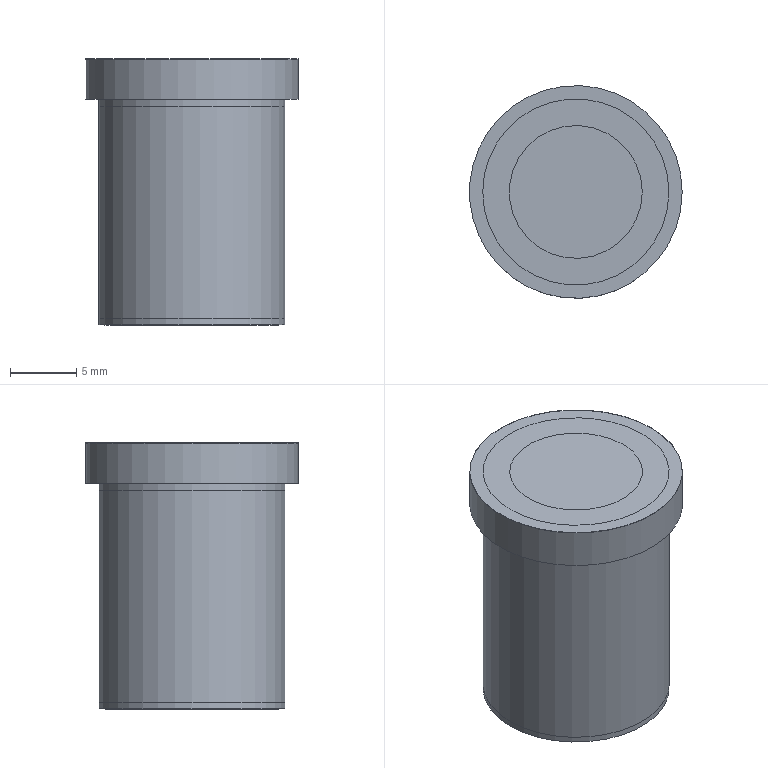Part | NX | features BREP 2 | 2 solids | 16 faces | box 16 x 16 x 20.03 mm | volume 4861 mm3 | plane 8 | cylinder 7 | cone 1 | commonest cylinder face diameters 14 x3 16 x2 10 x1 13.533 x1
STEP:
#1=CARTESIAN_POINT('',(8.,0.,-3.03));
#2=VERTEX_POINT('',#1);
#3=CARTESIAN_POINT('',(0.,0.,-3.03));
#4=DIRECTION('',(0.,0.,1.));
#5=DIRECTION('',(1.,0.,0.));
#6=AXIS2_PLACEMENT_3D('',#3,#4,#5);
#7=CIRCLE('',#6,8.);
#8=EDGE_CURVE('',#2,#2,#7,.T.);
#9=ORIENTED_EDGE('',*,*,#8,.T.);
#10=EDGE_LOOP('',(#9));
#11=FACE_BOUND('',#10,.T.);
#12=CARTESIAN_POINT('',(8.,0.,0.));
#13=VERTEX_POINT('',#12);
#14=CARTESIAN_POINT('',(0.,0.,0.));
#15=DIRECTION('',(0.,0.,1.));
#16=DIRECTION('',(1.,0.,0.));
#17=AXIS2_PLACEMENT_3D('',#14,#15,#16);
#18=CIRCLE('',#17,8.);
#19=EDGE_CURVE('',#13,#13,#18,.T.);
#20=ORIENTED_EDGE('',*,*,#19,.F.);
#21=EDGE_LOOP('',(#20));
#22=FACE_BOUND('',#21,.T.);
#23=CARTESIAN_POINT('',(0.,0.,-3.03));
#24=DIRECTION('',(0.,0.,1.));
#25=DIRECTION('',(-1.,0.,0.));
#26=AXIS2_PLACEMENT_3D('',#23,#24,#25);
#27=CYLINDRICAL_SURFACE('',#26,8.);
#28=ADVANCED_FACE('',(#11,#22),#27,.T.);
#29=CARTESIAN_POINT('',(-7.,0.,-3.03));
#30=VERTEX_POINT('',#29);
#31=CARTESIAN_POINT('',(0.,0.,-3.03));
#32=DIRECTION('',(0.,0.,-1.));
#33=DIRECTION('',(-1.,0.,0.));
#34=AXIS2_PLACEMENT_3D('',#31,#32,#33);
#35=CIRCLE('',#34,7.);
#36=EDGE_CURVE('',#30,#30,#35,.T.);
#37=ORIENTED_EDGE('',*,*,#36,.F.);
#38=EDGE_LOOP('',(#37));
#39=FACE_BOUND('',#38,.T.);
#40=ORIENTED_EDGE('',*,*,#8,.F.);
#41=EDGE_LOOP('',(#40));
#42=FACE_BOUND('',#41,.T.);
#43=CARTESIAN_POINT('',(0.,0.,-3.03));
#44=DIRECTION('',(0.,0.,1.));
#45=DIRECTION('',(-1.,0.,0.));
#46=AXIS2_PLACEMENT_3D('',#43,#44,#45);
#47=PLANE('',#46);
#48=ADVANCED_FACE('',(#39,#42),#47,.F.);
#49=ORIENTED_EDGE('',*,*,#19,.T.);
#50=EDGE_LOOP('',(#49));
#51=FACE_BOUND('',#50,.T.);
#52=CARTESIAN_POINT('',(0.,0.,0.));
#53=DIRECTION('',(0.,0.,1.));
#54=DIRECTION('',(-1.,0.,0.));
#55=AXIS2_PLACEMENT_3D('',#52,#53,#54);
#56=PLANE('',#55);
#57=ADVANCED_FACE('',(#51),#56,.T.);
#58=CARTESIAN_POINT('',(-7.,0.,-20.));
#59=VERTEX_POINT('',#58);
#60=CARTESIAN_POINT('',(0.,0.,-20.));
#61=DIRECTION('',(0.,0.,-1.));
#62=DIRECTION('',(-1.,0.,0.));
#63=AXIS2_PLACEMENT_3D('',#60,#61,#62);
#64=CIRCLE('',#63,7.);
#65=EDGE_CURVE('',#59,#59,#64,.T.);
#66=ORIENTED_EDGE('',*,*,#65,.T.);
#67=EDGE_LOOP('',(#66));
#68=FACE_BOUND('',#67,.T.);
#69=CARTESIAN_POINT('',(0.,0.,-20.));
#70=DIRECTION('',(0.,0.,-1.));
#71=DIRECTION('',(1.,0.,0.));
#72=AXIS2_PLACEMENT_3D('',#69,#70,#71);
#73=PLANE('',#72);
#74=ADVANCED_FACE('',(#68),#73,.T.);
#75=ORIENTED_EDGE('',*,*,#65,.F.);
#76=EDGE_LOOP('',(#75));
#77=FACE_BOUND('',#76,.T.);
#78=ORIENTED_EDGE('',*,*,#36,.T.);
#79=EDGE_LOOP('',(#78));
#80=FACE_BOUND('',#79,.T.);
#81=CARTESIAN_POINT('',(0.,0.,-3.03));
#82=DIRECTION('',(0.,0.,-1.));
#83=DIRECTION('',(1.,0.,0.));
#84=AXIS2_PLACEMENT_3D('',#81,#82,#83);
#85=CYLINDRICAL_SURFACE('',#84,7.);
#86=ADVANCED_FACE('',(#77,#80),#85,.T.);
#87=CLOSED_SHELL('',(#28,#48,#57,#74,#86));
#88=MANIFOLD_SOLID_BREP('',#87);
#89=CARTESIAN_POINT('',(-6.533,0.,-20.03));
#90=VERTEX_POINT('',#89);
#91=CARTESIAN_POINT('',(0.,0.,-20.03));
#92=DIRECTION('',(0.,0.,-1.));
#93=DIRECTION('',(-1.,0.,0.));
#94=AXIS2_PLACEMENT_3D('',#91,#92,#93);
#95=CIRCLE('',#94,6.533);
#96=EDGE_CURVE('',#90,#90,#95,.T.);
#97=ORIENTED_EDGE('',*,*,#96,.T.);
#98=EDGE_LOOP('',(#97));
#99=FACE_BOUND('',#98,.T.);
#100=CARTESIAN_POINT('',(5.,0.,-20.03));
#101=VERTEX_POINT('',#100);
#102=CARTESIAN_POINT('',(0.,0.,-20.03));
#103=DIRECTION('',(0.,0.,1.));
#104=DIRECTION('',(1.,0.,0.));
#105=AXIS2_PLACEMENT_3D('',#102,#103,#104);
#106=CIRCLE('',#105,5.);
#107=EDGE_CURVE('',#101,#101,#106,.T.);
#108=ORIENTED_EDGE('',*,*,#107,.T.);
#109=EDGE_LOOP('',(#108));
#110=FACE_BOUND('',#109,.T.);
#111=CARTESIAN_POINT('',(0.,0.,-20.03));
#112=DIRECTION('',(0.,0.,-1.));
#113=DIRECTION('',(1.,0.,0.));
#114=AXIS2_PLACEMENT_3D('',#111,#112,#113);
#115=PLANE('',#114);
#116=ADVANCED_FACE('',(#99,#110),#115,.T.);
#117=CARTESIAN_POINT('',(7.,0.,-0.026));
#118=VERTEX_POINT('',#117);
#119=CARTESIAN_POINT('',(0.,0.,-0.026));
#120=DIRECTION('',(0.,0.,1.));
#121=DIRECTION('',(1.,0.,0.));
#122=AXIS2_PLACEMENT_3D('',#119,#120,#121);
#123=CIRCLE('',#122,7.);
#124=EDGE_CURVE('',#118,#118,#123,.T.);
#125=ORIENTED_EDGE('',*,*,#124,.T.);
#126=EDGE_LOOP('',(#125));
#127=FACE_BOUND('',#126,.T.);
#128=CARTESIAN_POINT('',(5.,0.,-0.026));
#129=VERTEX_POINT('',#128);
#130=CARTESIAN_POINT('',(0.,0.,-0.026));
#131=DIRECTION('',(0.,0.,1.));
#132=DIRECTION('',(1.,0.,0.));
#133=AXIS2_PLACEMENT_3D('',#130,#131,#132);
#134=CIRCLE('',#133,5.);
#135=EDGE_CURVE('',#129,#129,#134,.T.);
#136=ORIENTED_EDGE('',*,*,#135,.F.);
#137=EDGE_LOOP('',(#136));
#138=FACE_BOUND('',#137,.T.);
#139=CARTESIAN_POINT('',(0.,0.,-0.026));
#140=DIRECTION('',(0.,0.,1.));
#141=DIRECTION('',(-1.,0.,0.));
#142=AXIS2_PLACEMENT_3D('',#139,#140,#141);
#143=PLANE('',#142);
#144=ADVANCED_FACE('',(#127,#138),#143,.T.);
#145=CARTESIAN_POINT('',(8.,0.,-3.03));
#146=VERTEX_POINT('',#145);
#147=CARTESIAN_POINT('',(0.,0.,-3.03));
#148=DIRECTION('',(0.,0.,1.));
#149=DIRECTION('',(1.,0.,0.));
#150=AXIS2_PLACEMENT_3D('',#147,#148,#149);
#151=CIRCLE('',#150,8.);
#152=EDGE_CURVE('',#146,#146,#151,.T.);
#153=ORIENTED_EDGE('',*,*,#152,.T.);
#154=EDGE_LOOP('',(#153));
#155=FACE_BOUND('',#154,.T.);
#156=CARTESIAN_POINT('',(8.,0.,-0.03));
#157=VERTEX_POINT('',#156);
#158=CARTESIAN_POINT('',(0.,0.,-0.03));
#159=DIRECTION('',(0.,0.,1.));
#160=DIRECTION('',(1.,0.,0.));
#161=AXIS2_PLACEMENT_3D('',#158,#159,#160);
#162=CIRCLE('',#161,8.);
#163=EDGE_CURVE('',#157,#157,#162,.T.);
#164=ORIENTED_EDGE('',*,*,#163,.F.);
#165=EDGE_LOOP('',(#164));
#166=FACE_BOUND('',#165,.T.);
#167=CARTESIAN_POINT('',(0.,0.,-3.03));
#168=DIRECTION('',(0.,0.,1.));
#169=DIRECTION('',(-1.,0.,0.));
#170=AXIS2_PLACEMENT_3D('',#167,#168,#169);
#171=CYLINDRICAL_SURFACE('',#170,8.);
#172=ADVANCED_FACE('',(#155,#166),#171,.T.);
#173=ORIENTED_EDGE('',*,*,#152,.F.);
#174=EDGE_LOOP('',(#173));
#175=FACE_BOUND('',#174,.T.);
#176=CARTESIAN_POINT('',(-6.767,0.,-3.03));
#177=VERTEX_POINT('',#176);
#178=CARTESIAN_POINT('',(0.,0.,-3.03));
#179=DIRECTION('',(0.,0.,-1.));
#180=DIRECTION('',(-1.,0.,0.));
#181=AXIS2_PLACEMENT_3D('',#178,#179,#180);
#182=CIRCLE('',#181,6.767);
#183=EDGE_CURVE('',#177,#177,#182,.T.);
#184=ORIENTED_EDGE('',*,*,#183,.F.);
#185=EDGE_LOOP('',(#184));
#186=FACE_BOUND('',#185,.T.);
#187=CARTESIAN_POINT('',(0.,0.,-3.03));
#188=DIRECTION('',(0.,0.,1.));
#189=DIRECTION('',(-1.,0.,0.));
#190=AXIS2_PLACEMENT_3D('',#187,#188,#189);
#191=PLANE('',#190);
#192=ADVANCED_FACE('',(#175,#186),#191,.F.);
#193=CARTESIAN_POINT('',(7.,0.,-0.03));
#194=VERTEX_POINT('',#193);
#195=CARTESIAN_POINT('',(0.,0.,-0.03));
#196=DIRECTION('',(0.,0.,1.));
#197=DIRECTION('',(1.,0.,0.));
#198=AXIS2_PLACEMENT_3D('',#195,#196,#197);
#199=CIRCLE('',#198,7.);
#200=EDGE_CURVE('',#194,#194,#199,.T.);
#201=ORIENTED_EDGE('',*,*,#200,.F.);
#202=EDGE_LOOP('',(#201));
#203=FACE_BOUND('',#202,.T.);
#204=ORIENTED_EDGE('',*,*,#163,.T.);
#205=EDGE_LOOP('',(#204));
#206=FACE_BOUND('',#205,.T.);
#207=CARTESIAN_POINT('',(0.,0.,-0.03));
#208=DIRECTION('',(0.,0.,1.));
#209=DIRECTION('',(-1.,0.,0.));
#210=AXIS2_PLACEMENT_3D('',#207,#208,#209);
#211=PLANE('',#210);
#212=ADVANCED_FACE('',(#203,#206),#211,.T.);
#213=CARTESIAN_POINT('',(-7.,0.,-19.563));
#214=VERTEX_POINT('',#213);
#215=CARTESIAN_POINT('',(0.,0.,-19.563));
#216=DIRECTION('',(0.,0.,1.));
#217=DIRECTION('',(-1.,0.,0.));
#218=AXIS2_PLACEMENT_3D('',#215,#216,#217);
#219=CIRCLE('',#218,7.);
#220=EDGE_CURVE('',#214,#214,#219,.T.);
#221=ORIENTED_EDGE('',*,*,#220,.T.);
#222=EDGE_LOOP('',(#221));
#223=FACE_BOUND('',#222,.T.);
#224=CARTESIAN_POINT('',(-7.,0.,-3.59));
#225=VERTEX_POINT('',#224);
#226=CARTESIAN_POINT('',(0.,0.,-3.59));
#227=DIRECTION('',(0.,0.,1.));
#228=DIRECTION('',(-1.,0.,0.));
#229=AXIS2_PLACEMENT_3D('',#226,#227,#228);
#230=CIRCLE('',#229,7.);
#231=EDGE_CURVE('',#225,#225,#230,.T.);
#232=ORIENTED_EDGE('',*,*,#231,.F.);
#233=EDGE_LOOP('',(#232));
#234=FACE_BOUND('',#233,.T.);
#235=CARTESIAN_POINT('',(0.,0.,-3.03));
#236=DIRECTION('',(0.,0.,-1.));
#237=DIRECTION('',(1.,0.,0.));
#238=AXIS2_PLACEMENT_3D('',#235,#236,#237);
#239=CYLINDRICAL_SURFACE('',#238,7.);
#240=ADVANCED_FACE('',(#223,#234),#239,.T.);
#241=ORIENTED_EDGE('',*,*,#124,.F.);
#242=EDGE_LOOP('',(#241));
#243=FACE_BOUND('',#242,.T.);
#244=ORIENTED_EDGE('',*,*,#200,.T.);
#245=EDGE_LOOP('',(#244));
#246=FACE_BOUND('',#245,.T.);
#247=CARTESIAN_POINT('',(0.,0.,-0.03));
#248=DIRECTION('',(0.,0.,1.));
#249=DIRECTION('',(-1.,0.,0.));
#250=AXIS2_PLACEMENT_3D('',#247,#248,#249);
#251=CYLINDRICAL_SURFACE('',#250,7.);
#252=ADVANCED_FACE('',(#243,#246),#251,.T.);
#253=ORIENTED_EDGE('',*,*,#135,.T.);
#254=EDGE_LOOP('',(#253));
#255=FACE_BOUND('',#254,.T.);
#256=ORIENTED_EDGE('',*,*,#107,.F.);
#257=EDGE_LOOP('',(#256));
#258=FACE_BOUND('',#257,.T.);
#259=CARTESIAN_POINT('',(0.,0.,-0.026));
#260=DIRECTION('',(0.,0.,-1.));
#261=DIRECTION('',(1.,0.,0.));
#262=AXIS2_PLACEMENT_3D('',#259,#260,#261);
#263=CYLINDRICAL_SURFACE('',#262,5.);
#264=ADVANCED_FACE('',(#255,#258),#263,.F.);
#265=CARTESIAN_POINT('',(-6.767,0.,-3.59));
#266=VERTEX_POINT('',#265);
#267=CARTESIAN_POINT('',(0.,0.,-3.59));
#268=DIRECTION('',(0.,0.,-1.));
#269=DIRECTION('',(-1.,0.,0.));
#270=AXIS2_PLACEMENT_3D('',#267,#268,#269);
#271=CIRCLE('',#270,6.767);
#272=EDGE_CURVE('',#266,#266,#271,.T.);
#273=ORIENTED_EDGE('',*,*,#272,.F.);
#274=EDGE_LOOP('',(#273));
#275=FACE_BOUND('',#274,.T.);
#276=ORIENTED_EDGE('',*,*,#183,.T.);
#277=EDGE_LOOP('',(#276));
#278=FACE_BOUND('',#277,.T.);
#279=CARTESIAN_POINT('',(0.,0.,-3.31));
#280=DIRECTION('',(0.,0.,-1.));
#281=DIRECTION('',(1.,0.,0.));
#282=AXIS2_PLACEMENT_3D('',#279,#280,#281);
#283=CYLINDRICAL_SURFACE('',#282,6.767);
#284=ADVANCED_FACE('',(#275,#278),#283,.T.);
#285=ORIENTED_EDGE('',*,*,#231,.T.);
#286=EDGE_LOOP('',(#285));
#287=FACE_BOUND('',#286,.T.);
#288=ORIENTED_EDGE('',*,*,#272,.T.);
#289=EDGE_LOOP('',(#288));
#290=FACE_BOUND('',#289,.T.);
#291=CARTESIAN_POINT('',(0.,0.,-3.59));
#292=DIRECTION('',(0.,0.,-1.));
#293=DIRECTION('',(1.,0.,0.));
#294=AXIS2_PLACEMENT_3D('',#291,#292,#293);
#295=PLANE('',#294);
#296=ADVANCED_FACE('',(#287,#290),#295,.F.);
#297=ORIENTED_EDGE('',*,*,#220,.F.);
#298=EDGE_LOOP('',(#297));
#299=FACE_BOUND('',#298,.T.);
#300=ORIENTED_EDGE('',*,*,#96,.F.);
#301=EDGE_LOOP('',(#300));
#302=FACE_BOUND('',#301,.T.);
#303=CARTESIAN_POINT('',(0.,0.,-20.03));
#304=DIRECTION('',(0.,0.,1.));
#305=DIRECTION('',(-1.,0.,0.));
#306=AXIS2_PLACEMENT_3D('',#303,#304,#305);
#307=CONICAL_SURFACE('',#306,6.533,0.7854);
#308=ADVANCED_FACE('',(#299,#302),#307,.T.);
#309=CLOSED_SHELL('',(#116,#144,#172,#192,#212,#240,#252,#264,#284,#296,#308));
#310=MANIFOLD_SOLID_BREP('',#309);
#311=(LENGTH_UNIT()NAMED_UNIT(*)SI_UNIT(.MILLI.,.METRE.));
#312=UNCERTAINTY_MEASURE_WITH_UNIT(LENGTH_MEASURE(0.00001),#311,'','');
#313=(NAMED_UNIT(*)PLANE_ANGLE_UNIT()SI_UNIT($,.RADIAN.));
#314=(NAMED_UNIT(*)SI_UNIT($,.STERADIAN.)SOLID_ANGLE_UNIT());
#315=(GEOMETRIC_REPRESENTATION_CONTEXT(3)GLOBAL_UNCERTAINTY_ASSIGNED_CONTEXT((#312))GLOBAL_UNIT_ASSIGNED_CONTEXT((#311,#313,#314))REPRESENTATION_CONTEXT('',''));
#316=ADVANCED_BREP_SHAPE_REPRESENTATION('',(#88,#310),#315);